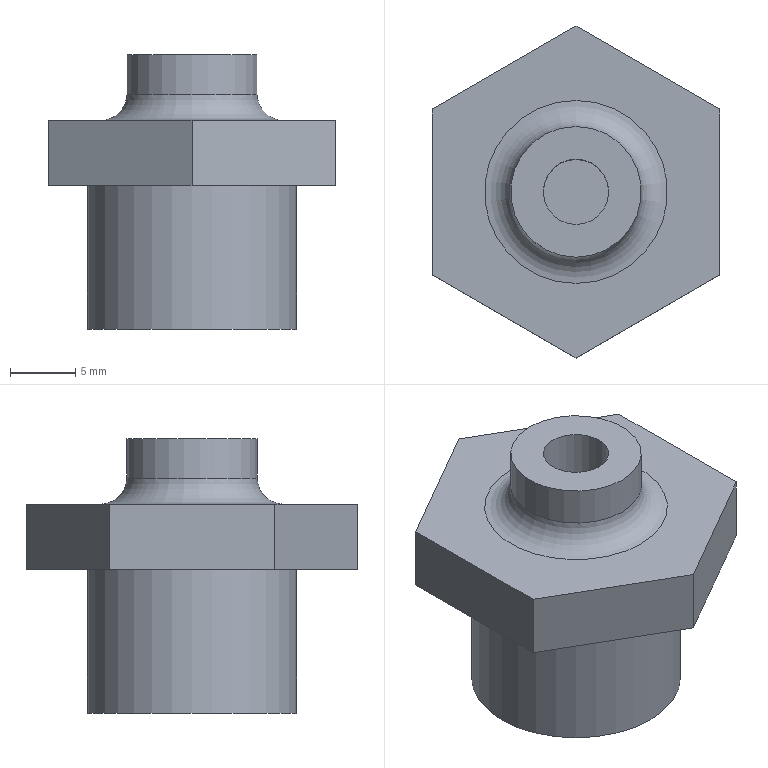Part | STEP file | 1-56.7 | 1 solid | 15 faces | box 22 x 25.403 x 21 mm | volume 4474 mm3 | plane 11 | cylinder 3 | torus 1 | commonest cylinder face diameters 5 x1 10 x1 16 x1
STEP:
#1=CARTESIAN_POINT('',(0.,0.,0.));
#2=DIRECTION('',(0.,0.,1.));
#3=DIRECTION('',(1.,0.,0.));
#4=AXIS2_PLACEMENT_3D('',#1,#2,#3);
#5=CARTESIAN_POINT('',(0.,8.,-11.));
#6=VERTEX_POINT('',#5);
#7=CARTESIAN_POINT('',(0.,0.,-11.));
#8=DIRECTION('',(0.,0.,1.));
#9=DIRECTION('',(0.,1.,0.));
#10=AXIS2_PLACEMENT_3D('',#7,#8,#9);
#11=CIRCLE('',#10,8.);
#12=CARTESIAN_POINT('',(0.,-2.144,-11.));
#13=DIRECTION('',(0.,0.,1.));
#14=DIRECTION('',(1.,0.,0.));
#15=AXIS2_PLACEMENT_3D('',#12,#13,#14);
#16=PLANE('',#15);
#17=CARTESIAN_POINT('',(0.,2.144));
#18=DIRECTION('',(0.,1.));
#19=AXIS2_PLACEMENT_2D('',#17,#18);
#20=CIRCLE('',#19,8.);
#21=(GEOMETRIC_REPRESENTATION_CONTEXT(2)PARAMETRIC_REPRESENTATION_CONTEXT()REPRESENTATION_CONTEXT('',''));
#22=DEFINITIONAL_REPRESENTATION('',(#20),#21);
#23=PCURVE('',#16,#22);
#24=CARTESIAN_POINT('',(0.,0.,0.));
#25=DIRECTION('',(0.,0.,-1.));
#26=DIRECTION('',(0.,1.,0.));
#27=AXIS2_PLACEMENT_3D('',#24,#25,#26);
#28=CYLINDRICAL_SURFACE('',#27,8.);
#29=CARTESIAN_POINT('',(6.283,11.));
#30=DIRECTION('',(-1.,0.));
#31=VECTOR('',#30,1.);
#32=LINE('',#29,#31);
#33=(GEOMETRIC_REPRESENTATION_CONTEXT(2)PARAMETRIC_REPRESENTATION_CONTEXT()REPRESENTATION_CONTEXT('',''));
#34=DEFINITIONAL_REPRESENTATION('',(#32),#33);
#35=PCURVE('',#28,#34);
#36=SURFACE_CURVE('',#11,(#23,#35),.PCURVE_S1.);
#37=EDGE_CURVE('',#6,#6,#36,.T.);
#38=ORIENTED_EDGE('',*,*,#37,.T.);
#39=EDGE_LOOP('',(#38));
#40=FACE_BOUND('',#39,.F.);
#41=ADVANCED_FACE('',(#40),#16,.F.);
#42=CARTESIAN_POINT('',(0.,8.,0.));
#43=VERTEX_POINT('',#42);
#44=CARTESIAN_POINT('',(0.,8.,0.));
#45=DIRECTION('',(0.,0.,-1.));
#46=VECTOR('',#45,1.);
#47=LINE('',#44,#46);
#48=CARTESIAN_POINT('',(6.283,0.));
#49=DIRECTION('',(0.,1.));
#50=VECTOR('',#49,1.);
#51=LINE('',#48,#50);
#52=(GEOMETRIC_REPRESENTATION_CONTEXT(2)PARAMETRIC_REPRESENTATION_CONTEXT()REPRESENTATION_CONTEXT('',''));
#53=DEFINITIONAL_REPRESENTATION('',(#51),#52);
#54=PCURVE('',#28,#53);
#55=CARTESIAN_POINT('',(0.,0.));
#56=DIRECTION('',(0.,1.));
#57=VECTOR('',#56,1.);
#58=LINE('',#55,#57);
#59=(GEOMETRIC_REPRESENTATION_CONTEXT(2)PARAMETRIC_REPRESENTATION_CONTEXT()REPRESENTATION_CONTEXT('',''));
#60=DEFINITIONAL_REPRESENTATION('',(#58),#59);
#61=PCURVE('',#28,#60);
#62=SEAM_CURVE('',#47,(#54,#61),.PCURVE_S1.);
#63=EDGE_CURVE('',#43,#6,#62,.T.);
#64=ORIENTED_EDGE('',*,*,#63,.T.);
#65=ORIENTED_EDGE('',*,*,#37,.T.);
#66=ORIENTED_EDGE('',*,*,#63,.F.);
#67=CARTESIAN_POINT('',(0.,0.,0.));
#68=DIRECTION('',(0.,0.,1.));
#69=DIRECTION('',(0.,1.,0.));
#70=AXIS2_PLACEMENT_3D('',#67,#68,#69);
#71=CIRCLE('',#70,8.);
#72=CARTESIAN_POINT('',(6.283,0.));
#73=DIRECTION('',(-1.,0.));
#74=VECTOR('',#73,1.);
#75=LINE('',#72,#74);
#76=(GEOMETRIC_REPRESENTATION_CONTEXT(2)PARAMETRIC_REPRESENTATION_CONTEXT()REPRESENTATION_CONTEXT('',''));
#77=DEFINITIONAL_REPRESENTATION('',(#75),#76);
#78=PCURVE('',#28,#77);
#79=CARTESIAN_POINT('',(1.702,0.,0.));
#80=DIRECTION('',(0.,0.,-1.));
#81=DIRECTION('',(1.,0.,0.));
#82=AXIS2_PLACEMENT_3D('',#79,#80,#81);
#83=PLANE('',#82);
#84=CARTESIAN_POINT('',(-1.702,-8.));
#85=CARTESIAN_POINT('',(-15.558,-8.));
#86=CARTESIAN_POINT('',(-8.63,4.));
#87=CARTESIAN_POINT('',(-1.702,16.));
#88=CARTESIAN_POINT('',(5.226,4.));
#89=CARTESIAN_POINT('',(12.155,-8.));
#90=CARTESIAN_POINT('',(-1.702,-8.));
#91=(BOUNDED_CURVE()B_SPLINE_CURVE(2,(#84,#85,#86,#87,#88,#89,#90),.UNSPECIFIED.,.T.,.F.)B_SPLINE_CURVE_WITH_KNOTS((1,2,2,2,2,1),(-2.094,0.,2.094,4.189,6.283,8.378),.UNSPECIFIED.)CURVE()GEOMETRIC_REPRESENTATION_ITEM()RATIONAL_B_SPLINE_CURVE((1.,0.5,1.,0.5,1.,0.5,1.))REPRESENTATION_ITEM(''));
#92=(GEOMETRIC_REPRESENTATION_CONTEXT(2)PARAMETRIC_REPRESENTATION_CONTEXT()REPRESENTATION_CONTEXT('',''));
#93=DEFINITIONAL_REPRESENTATION('',(#91),#92);
#94=PCURVE('',#83,#93);
#95=SURFACE_CURVE('',#71,(#78,#94),.PCURVE_S1.);
#96=EDGE_CURVE('',#43,#43,#95,.T.);
#97=ORIENTED_EDGE('',*,*,#96,.F.);
#98=EDGE_LOOP('',(#64,#65,#66,#97));
#99=FACE_BOUND('',#98,.T.);
#100=ADVANCED_FACE('',(#99),#28,.T.);
#101=CARTESIAN_POINT('',(-11.,-6.351,0.));
#102=VERTEX_POINT('',#101);
#103=CARTESIAN_POINT('',(-11.,6.351,0.));
#104=VERTEX_POINT('',#103);
#105=CARTESIAN_POINT('',(-11.,-6.351,0.));
#106=DIRECTION('',(0.,1.,0.));
#107=VECTOR('',#106,1.);
#108=LINE('',#105,#107);
#109=CARTESIAN_POINT('',(-12.702,6.351));
#110=DIRECTION('',(0.,-1.));
#111=VECTOR('',#110,1.);
#112=LINE('',#109,#111);
#113=(GEOMETRIC_REPRESENTATION_CONTEXT(2)PARAMETRIC_REPRESENTATION_CONTEXT()REPRESENTATION_CONTEXT('',''));
#114=DEFINITIONAL_REPRESENTATION('',(#112),#113);
#115=PCURVE('',#83,#114);
#116=CARTESIAN_POINT('',(-11.,0.,2.5));
#117=DIRECTION('',(1.,0.,0.));
#118=DIRECTION('',(0.,1.,0.));
#119=AXIS2_PLACEMENT_3D('',#116,#117,#118);
#120=PLANE('',#119);
#121=CARTESIAN_POINT('',(-6.351,-2.5));
#122=DIRECTION('',(1.,0.));
#123=VECTOR('',#122,1.);
#124=LINE('',#121,#123);
#125=(GEOMETRIC_REPRESENTATION_CONTEXT(2)PARAMETRIC_REPRESENTATION_CONTEXT()REPRESENTATION_CONTEXT('',''));
#126=DEFINITIONAL_REPRESENTATION('',(#124),#125);
#127=PCURVE('',#120,#126);
#128=SURFACE_CURVE('',#108,(#115,#127),.PCURVE_S1.);
#129=EDGE_CURVE('',#102,#104,#128,.T.);
#130=ORIENTED_EDGE('',*,*,#129,.T.);
#131=CARTESIAN_POINT('',(0.,12.702,0.));
#132=VERTEX_POINT('',#131);
#133=CARTESIAN_POINT('',(-11.,6.351,0.));
#134=DIRECTION('',(0.866,0.5,0.));
#135=VECTOR('',#134,1.);
#136=LINE('',#133,#135);
#137=CARTESIAN_POINT('',(-12.702,-6.351));
#138=DIRECTION('',(0.866,-0.5));
#139=VECTOR('',#138,1.);
#140=LINE('',#137,#139);
#141=(GEOMETRIC_REPRESENTATION_CONTEXT(2)PARAMETRIC_REPRESENTATION_CONTEXT()REPRESENTATION_CONTEXT('',''));
#142=DEFINITIONAL_REPRESENTATION('',(#140),#141);
#143=PCURVE('',#83,#142);
#144=CARTESIAN_POINT('',(-5.5,9.526,2.5));
#145=DIRECTION('',(0.5,-0.866,0.));
#146=DIRECTION('',(0.866,0.5,0.));
#147=AXIS2_PLACEMENT_3D('',#144,#145,#146);
#148=PLANE('',#147);
#149=CARTESIAN_POINT('',(-6.351,-2.5));
#150=DIRECTION('',(1.,0.));
#151=VECTOR('',#150,1.);
#152=LINE('',#149,#151);
#153=(GEOMETRIC_REPRESENTATION_CONTEXT(2)PARAMETRIC_REPRESENTATION_CONTEXT()REPRESENTATION_CONTEXT('',''));
#154=DEFINITIONAL_REPRESENTATION('',(#152),#153);
#155=PCURVE('',#148,#154);
#156=SURFACE_CURVE('',#136,(#143,#155),.PCURVE_S1.);
#157=EDGE_CURVE('',#104,#132,#156,.T.);
#158=ORIENTED_EDGE('',*,*,#157,.T.);
#159=CARTESIAN_POINT('',(11.,6.351,0.));
#160=VERTEX_POINT('',#159);
#161=CARTESIAN_POINT('',(0.,12.702,0.));
#162=DIRECTION('',(0.866,-0.5,0.));
#163=VECTOR('',#162,1.);
#164=LINE('',#161,#163);
#165=CARTESIAN_POINT('',(-1.702,-12.702));
#166=DIRECTION('',(0.866,0.5));
#167=VECTOR('',#166,1.);
#168=LINE('',#165,#167);
#169=(GEOMETRIC_REPRESENTATION_CONTEXT(2)PARAMETRIC_REPRESENTATION_CONTEXT()REPRESENTATION_CONTEXT('',''));
#170=DEFINITIONAL_REPRESENTATION('',(#168),#169);
#171=PCURVE('',#83,#170);
#172=CARTESIAN_POINT('',(5.5,9.526,2.5));
#173=DIRECTION('',(-0.5,-0.866,0.));
#174=DIRECTION('',(0.866,-0.5,0.));
#175=AXIS2_PLACEMENT_3D('',#172,#173,#174);
#176=PLANE('',#175);
#177=CARTESIAN_POINT('',(-6.351,-2.5));
#178=DIRECTION('',(1.,0.));
#179=VECTOR('',#178,1.);
#180=LINE('',#177,#179);
#181=(GEOMETRIC_REPRESENTATION_CONTEXT(2)PARAMETRIC_REPRESENTATION_CONTEXT()REPRESENTATION_CONTEXT('',''));
#182=DEFINITIONAL_REPRESENTATION('',(#180),#181);
#183=PCURVE('',#176,#182);
#184=SURFACE_CURVE('',#164,(#171,#183),.PCURVE_S1.);
#185=EDGE_CURVE('',#132,#160,#184,.T.);
#186=ORIENTED_EDGE('',*,*,#185,.T.);
#187=CARTESIAN_POINT('',(11.,-6.351,0.));
#188=VERTEX_POINT('',#187);
#189=CARTESIAN_POINT('',(11.,6.351,0.));
#190=DIRECTION('',(0.,-1.,0.));
#191=VECTOR('',#190,1.);
#192=LINE('',#189,#191);
#193=CARTESIAN_POINT('',(9.298,-6.351));
#194=DIRECTION('',(0.,1.));
#195=VECTOR('',#194,1.);
#196=LINE('',#193,#195);
#197=(GEOMETRIC_REPRESENTATION_CONTEXT(2)PARAMETRIC_REPRESENTATION_CONTEXT()REPRESENTATION_CONTEXT('',''));
#198=DEFINITIONAL_REPRESENTATION('',(#196),#197);
#199=PCURVE('',#83,#198);
#200=CARTESIAN_POINT('',(11.,0.,2.5));
#201=DIRECTION('',(-1.,0.,0.));
#202=DIRECTION('',(0.,-1.,0.));
#203=AXIS2_PLACEMENT_3D('',#200,#201,#202);
#204=PLANE('',#203);
#205=CARTESIAN_POINT('',(-6.351,-2.5));
#206=DIRECTION('',(1.,0.));
#207=VECTOR('',#206,1.);
#208=LINE('',#205,#207);
#209=(GEOMETRIC_REPRESENTATION_CONTEXT(2)PARAMETRIC_REPRESENTATION_CONTEXT()REPRESENTATION_CONTEXT('',''));
#210=DEFINITIONAL_REPRESENTATION('',(#208),#209);
#211=PCURVE('',#204,#210);
#212=SURFACE_CURVE('',#192,(#199,#211),.PCURVE_S1.);
#213=EDGE_CURVE('',#160,#188,#212,.T.);
#214=ORIENTED_EDGE('',*,*,#213,.T.);
#215=CARTESIAN_POINT('',(0.,-12.702,0.));
#216=VERTEX_POINT('',#215);
#217=CARTESIAN_POINT('',(11.,-6.351,0.));
#218=DIRECTION('',(-0.866,-0.5,0.));
#219=VECTOR('',#218,1.);
#220=LINE('',#217,#219);
#221=CARTESIAN_POINT('',(9.298,6.351));
#222=DIRECTION('',(-0.866,0.5));
#223=VECTOR('',#222,1.);
#224=LINE('',#221,#223);
#225=(GEOMETRIC_REPRESENTATION_CONTEXT(2)PARAMETRIC_REPRESENTATION_CONTEXT()REPRESENTATION_CONTEXT('',''));
#226=DEFINITIONAL_REPRESENTATION('',(#224),#225);
#227=PCURVE('',#83,#226);
#228=CARTESIAN_POINT('',(5.5,-9.526,2.5));
#229=DIRECTION('',(-0.5,0.866,0.));
#230=DIRECTION('',(-0.866,-0.5,0.));
#231=AXIS2_PLACEMENT_3D('',#228,#229,#230);
#232=PLANE('',#231);
#233=CARTESIAN_POINT('',(-6.351,-2.5));
#234=DIRECTION('',(1.,0.));
#235=VECTOR('',#234,1.);
#236=LINE('',#233,#235);
#237=(GEOMETRIC_REPRESENTATION_CONTEXT(2)PARAMETRIC_REPRESENTATION_CONTEXT()REPRESENTATION_CONTEXT('',''));
#238=DEFINITIONAL_REPRESENTATION('',(#236),#237);
#239=PCURVE('',#232,#238);
#240=SURFACE_CURVE('',#220,(#227,#239),.PCURVE_S1.);
#241=EDGE_CURVE('',#188,#216,#240,.T.);
#242=ORIENTED_EDGE('',*,*,#241,.T.);
#243=CARTESIAN_POINT('',(0.,-12.702,0.));
#244=DIRECTION('',(-0.866,0.5,0.));
#245=VECTOR('',#244,1.);
#246=LINE('',#243,#245);
#247=CARTESIAN_POINT('',(-1.702,12.702));
#248=DIRECTION('',(-0.866,-0.5));
#249=VECTOR('',#248,1.);
#250=LINE('',#247,#249);
#251=(GEOMETRIC_REPRESENTATION_CONTEXT(2)PARAMETRIC_REPRESENTATION_CONTEXT()REPRESENTATION_CONTEXT('',''));
#252=DEFINITIONAL_REPRESENTATION('',(#250),#251);
#253=PCURVE('',#83,#252);
#254=CARTESIAN_POINT('',(-5.5,-9.526,2.5));
#255=DIRECTION('',(0.5,0.866,0.));
#256=DIRECTION('',(-0.866,0.5,0.));
#257=AXIS2_PLACEMENT_3D('',#254,#255,#256);
#258=PLANE('',#257);
#259=CARTESIAN_POINT('',(-6.351,-2.5));
#260=DIRECTION('',(1.,0.));
#261=VECTOR('',#260,1.);
#262=LINE('',#259,#261);
#263=(GEOMETRIC_REPRESENTATION_CONTEXT(2)PARAMETRIC_REPRESENTATION_CONTEXT()REPRESENTATION_CONTEXT('',''));
#264=DEFINITIONAL_REPRESENTATION('',(#262),#263);
#265=PCURVE('',#258,#264);
#266=SURFACE_CURVE('',#246,(#253,#265),.PCURVE_S1.);
#267=EDGE_CURVE('',#216,#102,#266,.T.);
#268=ORIENTED_EDGE('',*,*,#267,.T.);
#269=EDGE_LOOP('',(#130,#158,#186,#214,#242,#268));
#270=FACE_BOUND('',#269,.T.);
#271=ORIENTED_EDGE('',*,*,#96,.T.);
#272=EDGE_LOOP('',(#271));
#273=FACE_BOUND('',#272,.T.);
#274=ADVANCED_FACE('',(#270,#273),#83,.T.);
#275=ORIENTED_EDGE('',*,*,#129,.T.);
#276=CARTESIAN_POINT('',(-11.,6.351,5.));
#277=VERTEX_POINT('',#276);
#278=CARTESIAN_POINT('',(-11.,6.351,0.));
#279=DIRECTION('',(0.,0.,1.));
#280=VECTOR('',#279,1.);
#281=LINE('',#278,#280);
#282=CARTESIAN_POINT('',(6.351,-2.5));
#283=DIRECTION('',(0.,1.));
#284=VECTOR('',#283,1.);
#285=LINE('',#282,#284);
#286=(GEOMETRIC_REPRESENTATION_CONTEXT(2)PARAMETRIC_REPRESENTATION_CONTEXT()REPRESENTATION_CONTEXT('',''));
#287=DEFINITIONAL_REPRESENTATION('',(#285),#286);
#288=PCURVE('',#120,#287);
#289=CARTESIAN_POINT('',(-6.351,-2.5));
#290=DIRECTION('',(0.,1.));
#291=VECTOR('',#290,1.);
#292=LINE('',#289,#291);
#293=(GEOMETRIC_REPRESENTATION_CONTEXT(2)PARAMETRIC_REPRESENTATION_CONTEXT()REPRESENTATION_CONTEXT('',''));
#294=DEFINITIONAL_REPRESENTATION('',(#292),#293);
#295=PCURVE('',#148,#294);
#296=SURFACE_CURVE('',#281,(#288,#295),.PCURVE_S1.);
#297=EDGE_CURVE('',#104,#277,#296,.T.);
#298=ORIENTED_EDGE('',*,*,#297,.T.);
#299=CARTESIAN_POINT('',(-11.,-6.351,5.));
#300=VERTEX_POINT('',#299);
#301=CARTESIAN_POINT('',(-11.,-6.351,5.));
#302=DIRECTION('',(0.,1.,0.));
#303=VECTOR('',#302,1.);
#304=LINE('',#301,#303);
#305=CARTESIAN_POINT('',(-6.351,2.5));
#306=DIRECTION('',(1.,0.));
#307=VECTOR('',#306,1.);
#308=LINE('',#305,#307);
#309=(GEOMETRIC_REPRESENTATION_CONTEXT(2)PARAMETRIC_REPRESENTATION_CONTEXT()REPRESENTATION_CONTEXT('',''));
#310=DEFINITIONAL_REPRESENTATION('',(#308),#309);
#311=PCURVE('',#120,#310);
#312=CARTESIAN_POINT('',(1.702,0.,5.));
#313=DIRECTION('',(0.,0.,-1.));
#314=DIRECTION('',(1.,0.,0.));
#315=AXIS2_PLACEMENT_3D('',#312,#313,#314);
#316=PLANE('',#315);
#317=CARTESIAN_POINT('',(-12.702,6.351));
#318=DIRECTION('',(0.,-1.));
#319=VECTOR('',#318,1.);
#320=LINE('',#317,#319);
#321=(GEOMETRIC_REPRESENTATION_CONTEXT(2)PARAMETRIC_REPRESENTATION_CONTEXT()REPRESENTATION_CONTEXT('',''));
#322=DEFINITIONAL_REPRESENTATION('',(#320),#321);
#323=PCURVE('',#316,#322);
#324=SURFACE_CURVE('',#304,(#311,#323),.PCURVE_S1.);
#325=EDGE_CURVE('',#300,#277,#324,.T.);
#326=ORIENTED_EDGE('',*,*,#325,.F.);
#327=CARTESIAN_POINT('',(-11.,-6.351,0.));
#328=DIRECTION('',(0.,0.,1.));
#329=VECTOR('',#328,1.);
#330=LINE('',#327,#329);
#331=CARTESIAN_POINT('',(-6.351,-2.5));
#332=DIRECTION('',(0.,1.));
#333=VECTOR('',#332,1.);
#334=LINE('',#331,#333);
#335=(GEOMETRIC_REPRESENTATION_CONTEXT(2)PARAMETRIC_REPRESENTATION_CONTEXT()REPRESENTATION_CONTEXT('',''));
#336=DEFINITIONAL_REPRESENTATION('',(#334),#335);
#337=PCURVE('',#120,#336);
#338=CARTESIAN_POINT('',(6.351,-2.5));
#339=DIRECTION('',(0.,1.));
#340=VECTOR('',#339,1.);
#341=LINE('',#338,#340);
#342=(GEOMETRIC_REPRESENTATION_CONTEXT(2)PARAMETRIC_REPRESENTATION_CONTEXT()REPRESENTATION_CONTEXT('',''));
#343=DEFINITIONAL_REPRESENTATION('',(#341),#342);
#344=PCURVE('',#258,#343);
#345=SURFACE_CURVE('',#330,(#337,#344),.PCURVE_S1.);
#346=EDGE_CURVE('',#102,#300,#345,.T.);
#347=ORIENTED_EDGE('',*,*,#346,.F.);
#348=EDGE_LOOP('',(#275,#298,#326,#347));
#349=FACE_BOUND('',#348,.F.);
#350=ADVANCED_FACE('',(#349),#120,.F.);
#351=ORIENTED_EDGE('',*,*,#157,.T.);
#352=CARTESIAN_POINT('',(0.,12.702,5.));
#353=VERTEX_POINT('',#352);
#354=CARTESIAN_POINT('',(0.,12.702,0.));
#355=DIRECTION('',(0.,0.,1.));
#356=VECTOR('',#355,1.);
#357=LINE('',#354,#356);
#358=CARTESIAN_POINT('',(6.351,-2.5));
#359=DIRECTION('',(0.,1.));
#360=VECTOR('',#359,1.);
#361=LINE('',#358,#360);
#362=(GEOMETRIC_REPRESENTATION_CONTEXT(2)PARAMETRIC_REPRESENTATION_CONTEXT()REPRESENTATION_CONTEXT('',''));
#363=DEFINITIONAL_REPRESENTATION('',(#361),#362);
#364=PCURVE('',#148,#363);
#365=CARTESIAN_POINT('',(-6.351,-2.5));
#366=DIRECTION('',(0.,1.));
#367=VECTOR('',#366,1.);
#368=LINE('',#365,#367);
#369=(GEOMETRIC_REPRESENTATION_CONTEXT(2)PARAMETRIC_REPRESENTATION_CONTEXT()REPRESENTATION_CONTEXT('',''));
#370=DEFINITIONAL_REPRESENTATION('',(#368),#369);
#371=PCURVE('',#176,#370);
#372=SURFACE_CURVE('',#357,(#364,#371),.PCURVE_S1.);
#373=EDGE_CURVE('',#132,#353,#372,.T.);
#374=ORIENTED_EDGE('',*,*,#373,.T.);
#375=CARTESIAN_POINT('',(-11.,6.351,5.));
#376=DIRECTION('',(0.866,0.5,0.));
#377=VECTOR('',#376,1.);
#378=LINE('',#375,#377);
#379=CARTESIAN_POINT('',(-6.351,2.5));
#380=DIRECTION('',(1.,0.));
#381=VECTOR('',#380,1.);
#382=LINE('',#379,#381);
#383=(GEOMETRIC_REPRESENTATION_CONTEXT(2)PARAMETRIC_REPRESENTATION_CONTEXT()REPRESENTATION_CONTEXT('',''));
#384=DEFINITIONAL_REPRESENTATION('',(#382),#383);
#385=PCURVE('',#148,#384);
#386=CARTESIAN_POINT('',(-12.702,-6.351));
#387=DIRECTION('',(0.866,-0.5));
#388=VECTOR('',#387,1.);
#389=LINE('',#386,#388);
#390=(GEOMETRIC_REPRESENTATION_CONTEXT(2)PARAMETRIC_REPRESENTATION_CONTEXT()REPRESENTATION_CONTEXT('',''));
#391=DEFINITIONAL_REPRESENTATION('',(#389),#390);
#392=PCURVE('',#316,#391);
#393=SURFACE_CURVE('',#378,(#385,#392),.PCURVE_S1.);
#394=EDGE_CURVE('',#277,#353,#393,.T.);
#395=ORIENTED_EDGE('',*,*,#394,.F.);
#396=ORIENTED_EDGE('',*,*,#297,.F.);
#397=EDGE_LOOP('',(#351,#374,#395,#396));
#398=FACE_BOUND('',#397,.F.);
#399=ADVANCED_FACE('',(#398),#148,.F.);
#400=ORIENTED_EDGE('',*,*,#185,.T.);
#401=CARTESIAN_POINT('',(11.,6.351,5.));
#402=VERTEX_POINT('',#401);
#403=CARTESIAN_POINT('',(11.,6.351,0.));
#404=DIRECTION('',(0.,0.,1.));
#405=VECTOR('',#404,1.);
#406=LINE('',#403,#405);
#407=CARTESIAN_POINT('',(6.351,-2.5));
#408=DIRECTION('',(0.,1.));
#409=VECTOR('',#408,1.);
#410=LINE('',#407,#409);
#411=(GEOMETRIC_REPRESENTATION_CONTEXT(2)PARAMETRIC_REPRESENTATION_CONTEXT()REPRESENTATION_CONTEXT('',''));
#412=DEFINITIONAL_REPRESENTATION('',(#410),#411);
#413=PCURVE('',#176,#412);
#414=CARTESIAN_POINT('',(-6.351,-2.5));
#415=DIRECTION('',(0.,1.));
#416=VECTOR('',#415,1.);
#417=LINE('',#414,#416);
#418=(GEOMETRIC_REPRESENTATION_CONTEXT(2)PARAMETRIC_REPRESENTATION_CONTEXT()REPRESENTATION_CONTEXT('',''));
#419=DEFINITIONAL_REPRESENTATION('',(#417),#418);
#420=PCURVE('',#204,#419);
#421=SURFACE_CURVE('',#406,(#413,#420),.PCURVE_S1.);
#422=EDGE_CURVE('',#160,#402,#421,.T.);
#423=ORIENTED_EDGE('',*,*,#422,.T.);
#424=CARTESIAN_POINT('',(0.,12.702,5.));
#425=DIRECTION('',(0.866,-0.5,0.));
#426=VECTOR('',#425,1.);
#427=LINE('',#424,#426);
#428=CARTESIAN_POINT('',(-6.351,2.5));
#429=DIRECTION('',(1.,0.));
#430=VECTOR('',#429,1.);
#431=LINE('',#428,#430);
#432=(GEOMETRIC_REPRESENTATION_CONTEXT(2)PARAMETRIC_REPRESENTATION_CONTEXT()REPRESENTATION_CONTEXT('',''));
#433=DEFINITIONAL_REPRESENTATION('',(#431),#432);
#434=PCURVE('',#176,#433);
#435=CARTESIAN_POINT('',(-1.702,-12.702));
#436=DIRECTION('',(0.866,0.5));
#437=VECTOR('',#436,1.);
#438=LINE('',#435,#437);
#439=(GEOMETRIC_REPRESENTATION_CONTEXT(2)PARAMETRIC_REPRESENTATION_CONTEXT()REPRESENTATION_CONTEXT('',''));
#440=DEFINITIONAL_REPRESENTATION('',(#438),#439);
#441=PCURVE('',#316,#440);
#442=SURFACE_CURVE('',#427,(#434,#441),.PCURVE_S1.);
#443=EDGE_CURVE('',#353,#402,#442,.T.);
#444=ORIENTED_EDGE('',*,*,#443,.F.);
#445=ORIENTED_EDGE('',*,*,#373,.F.);
#446=EDGE_LOOP('',(#400,#423,#444,#445));
#447=FACE_BOUND('',#446,.F.);
#448=ADVANCED_FACE('',(#447),#176,.F.);
#449=ORIENTED_EDGE('',*,*,#213,.T.);
#450=CARTESIAN_POINT('',(11.,-6.351,5.));
#451=VERTEX_POINT('',#450);
#452=CARTESIAN_POINT('',(11.,-6.351,0.));
#453=DIRECTION('',(0.,0.,1.));
#454=VECTOR('',#453,1.);
#455=LINE('',#452,#454);
#456=CARTESIAN_POINT('',(6.351,-2.5));
#457=DIRECTION('',(0.,1.));
#458=VECTOR('',#457,1.);
#459=LINE('',#456,#458);
#460=(GEOMETRIC_REPRESENTATION_CONTEXT(2)PARAMETRIC_REPRESENTATION_CONTEXT()REPRESENTATION_CONTEXT('',''));
#461=DEFINITIONAL_REPRESENTATION('',(#459),#460);
#462=PCURVE('',#204,#461);
#463=CARTESIAN_POINT('',(-6.351,-2.5));
#464=DIRECTION('',(0.,1.));
#465=VECTOR('',#464,1.);
#466=LINE('',#463,#465);
#467=(GEOMETRIC_REPRESENTATION_CONTEXT(2)PARAMETRIC_REPRESENTATION_CONTEXT()REPRESENTATION_CONTEXT('',''));
#468=DEFINITIONAL_REPRESENTATION('',(#466),#467);
#469=PCURVE('',#232,#468);
#470=SURFACE_CURVE('',#455,(#462,#469),.PCURVE_S1.);
#471=EDGE_CURVE('',#188,#451,#470,.T.);
#472=ORIENTED_EDGE('',*,*,#471,.T.);
#473=CARTESIAN_POINT('',(11.,6.351,5.));
#474=DIRECTION('',(0.,-1.,0.));
#475=VECTOR('',#474,1.);
#476=LINE('',#473,#475);
#477=CARTESIAN_POINT('',(-6.351,2.5));
#478=DIRECTION('',(1.,0.));
#479=VECTOR('',#478,1.);
#480=LINE('',#477,#479);
#481=(GEOMETRIC_REPRESENTATION_CONTEXT(2)PARAMETRIC_REPRESENTATION_CONTEXT()REPRESENTATION_CONTEXT('',''));
#482=DEFINITIONAL_REPRESENTATION('',(#480),#481);
#483=PCURVE('',#204,#482);
#484=CARTESIAN_POINT('',(9.298,-6.351));
#485=DIRECTION('',(0.,1.));
#486=VECTOR('',#485,1.);
#487=LINE('',#484,#486);
#488=(GEOMETRIC_REPRESENTATION_CONTEXT(2)PARAMETRIC_REPRESENTATION_CONTEXT()REPRESENTATION_CONTEXT('',''));
#489=DEFINITIONAL_REPRESENTATION('',(#487),#488);
#490=PCURVE('',#316,#489);
#491=SURFACE_CURVE('',#476,(#483,#490),.PCURVE_S1.);
#492=EDGE_CURVE('',#402,#451,#491,.T.);
#493=ORIENTED_EDGE('',*,*,#492,.F.);
#494=ORIENTED_EDGE('',*,*,#422,.F.);
#495=EDGE_LOOP('',(#449,#472,#493,#494));
#496=FACE_BOUND('',#495,.F.);
#497=ADVANCED_FACE('',(#496),#204,.F.);
#498=ORIENTED_EDGE('',*,*,#241,.T.);
#499=CARTESIAN_POINT('',(0.,-12.702,5.));
#500=VERTEX_POINT('',#499);
#501=CARTESIAN_POINT('',(0.,-12.702,0.));
#502=DIRECTION('',(0.,0.,1.));
#503=VECTOR('',#502,1.);
#504=LINE('',#501,#503);
#505=CARTESIAN_POINT('',(6.351,-2.5));
#506=DIRECTION('',(0.,1.));
#507=VECTOR('',#506,1.);
#508=LINE('',#505,#507);
#509=(GEOMETRIC_REPRESENTATION_CONTEXT(2)PARAMETRIC_REPRESENTATION_CONTEXT()REPRESENTATION_CONTEXT('',''));
#510=DEFINITIONAL_REPRESENTATION('',(#508),#509);
#511=PCURVE('',#232,#510);
#512=CARTESIAN_POINT('',(-6.351,-2.5));
#513=DIRECTION('',(0.,1.));
#514=VECTOR('',#513,1.);
#515=LINE('',#512,#514);
#516=(GEOMETRIC_REPRESENTATION_CONTEXT(2)PARAMETRIC_REPRESENTATION_CONTEXT()REPRESENTATION_CONTEXT('',''));
#517=DEFINITIONAL_REPRESENTATION('',(#515),#516);
#518=PCURVE('',#258,#517);
#519=SURFACE_CURVE('',#504,(#511,#518),.PCURVE_S1.);
#520=EDGE_CURVE('',#216,#500,#519,.T.);
#521=ORIENTED_EDGE('',*,*,#520,.T.);
#522=CARTESIAN_POINT('',(11.,-6.351,5.));
#523=DIRECTION('',(-0.866,-0.5,0.));
#524=VECTOR('',#523,1.);
#525=LINE('',#522,#524);
#526=CARTESIAN_POINT('',(-6.351,2.5));
#527=DIRECTION('',(1.,0.));
#528=VECTOR('',#527,1.);
#529=LINE('',#526,#528);
#530=(GEOMETRIC_REPRESENTATION_CONTEXT(2)PARAMETRIC_REPRESENTATION_CONTEXT()REPRESENTATION_CONTEXT('',''));
#531=DEFINITIONAL_REPRESENTATION('',(#529),#530);
#532=PCURVE('',#232,#531);
#533=CARTESIAN_POINT('',(9.298,6.351));
#534=DIRECTION('',(-0.866,0.5));
#535=VECTOR('',#534,1.);
#536=LINE('',#533,#535);
#537=(GEOMETRIC_REPRESENTATION_CONTEXT(2)PARAMETRIC_REPRESENTATION_CONTEXT()REPRESENTATION_CONTEXT('',''));
#538=DEFINITIONAL_REPRESENTATION('',(#536),#537);
#539=PCURVE('',#316,#538);
#540=SURFACE_CURVE('',#525,(#532,#539),.PCURVE_S1.);
#541=EDGE_CURVE('',#451,#500,#540,.T.);
#542=ORIENTED_EDGE('',*,*,#541,.F.);
#543=ORIENTED_EDGE('',*,*,#471,.F.);
#544=EDGE_LOOP('',(#498,#521,#542,#543));
#545=FACE_BOUND('',#544,.F.);
#546=ADVANCED_FACE('',(#545),#232,.F.);
#547=ORIENTED_EDGE('',*,*,#267,.T.);
#548=ORIENTED_EDGE('',*,*,#346,.T.);
#549=CARTESIAN_POINT('',(0.,-12.702,5.));
#550=DIRECTION('',(-0.866,0.5,0.));
#551=VECTOR('',#550,1.);
#552=LINE('',#549,#551);
#553=CARTESIAN_POINT('',(-6.351,2.5));
#554=DIRECTION('',(1.,0.));
#555=VECTOR('',#554,1.);
#556=LINE('',#553,#555);
#557=(GEOMETRIC_REPRESENTATION_CONTEXT(2)PARAMETRIC_REPRESENTATION_CONTEXT()REPRESENTATION_CONTEXT('',''));
#558=DEFINITIONAL_REPRESENTATION('',(#556),#557);
#559=PCURVE('',#258,#558);
#560=CARTESIAN_POINT('',(-1.702,12.702));
#561=DIRECTION('',(-0.866,-0.5));
#562=VECTOR('',#561,1.);
#563=LINE('',#560,#562);
#564=(GEOMETRIC_REPRESENTATION_CONTEXT(2)PARAMETRIC_REPRESENTATION_CONTEXT()REPRESENTATION_CONTEXT('',''));
#565=DEFINITIONAL_REPRESENTATION('',(#563),#564);
#566=PCURVE('',#316,#565);
#567=SURFACE_CURVE('',#552,(#559,#566),.PCURVE_S1.);
#568=EDGE_CURVE('',#500,#300,#567,.T.);
#569=ORIENTED_EDGE('',*,*,#568,.F.);
#570=ORIENTED_EDGE('',*,*,#520,.F.);
#571=EDGE_LOOP('',(#547,#548,#569,#570));
#572=FACE_BOUND('',#571,.F.);
#573=ADVANCED_FACE('',(#572),#258,.F.);
#574=CARTESIAN_POINT('',(0.,5.,10.));
#575=VERTEX_POINT('',#574);
#576=CARTESIAN_POINT('',(0.,0.,10.));
#577=DIRECTION('',(0.,0.,1.));
#578=DIRECTION('',(0.,1.,0.));
#579=AXIS2_PLACEMENT_3D('',#576,#577,#578);
#580=CIRCLE('',#579,5.);
#581=CARTESIAN_POINT('',(0.,-1.34,10.));
#582=DIRECTION('',(0.,0.,1.));
#583=DIRECTION('',(1.,0.,0.));
#584=AXIS2_PLACEMENT_3D('',#581,#582,#583);
#585=PLANE('',#584);
#586=CARTESIAN_POINT('',(0.,1.34));
#587=DIRECTION('',(0.,1.));
#588=AXIS2_PLACEMENT_2D('',#586,#587);
#589=CIRCLE('',#588,5.);
#590=(GEOMETRIC_REPRESENTATION_CONTEXT(2)PARAMETRIC_REPRESENTATION_CONTEXT()REPRESENTATION_CONTEXT('',''));
#591=DEFINITIONAL_REPRESENTATION('',(#589),#590);
#592=PCURVE('',#585,#591);
#593=CARTESIAN_POINT('',(0.,0.,5.));
#594=DIRECTION('',(0.,0.,1.));
#595=DIRECTION('',(0.,1.,0.));
#596=AXIS2_PLACEMENT_3D('',#593,#594,#595);
#597=CYLINDRICAL_SURFACE('',#596,5.);
#598=CARTESIAN_POINT('',(0.,5.));
#599=DIRECTION('',(1.,0.));
#600=VECTOR('',#599,1.);
#601=LINE('',#598,#600);
#602=(GEOMETRIC_REPRESENTATION_CONTEXT(2)PARAMETRIC_REPRESENTATION_CONTEXT()REPRESENTATION_CONTEXT('',''));
#603=DEFINITIONAL_REPRESENTATION('',(#601),#602);
#604=PCURVE('',#597,#603);
#605=SURFACE_CURVE('',#580,(#592,#604),.PCURVE_S1.);
#606=EDGE_CURVE('',#575,#575,#605,.T.);
#607=ORIENTED_EDGE('',*,*,#606,.T.);
#608=EDGE_LOOP('',(#607));
#609=FACE_BOUND('',#608,.T.);
#610=CARTESIAN_POINT('',(0.,2.5,10.));
#611=VERTEX_POINT('',#610);
#612=CARTESIAN_POINT('',(0.,0.,10.));
#613=DIRECTION('',(0.,0.,1.));
#614=DIRECTION('',(0.,1.,0.));
#615=AXIS2_PLACEMENT_3D('',#612,#613,#614);
#616=CIRCLE('',#615,2.5);
#617=CARTESIAN_POINT('',(0.,1.34));
#618=DIRECTION('',(0.,1.));
#619=AXIS2_PLACEMENT_2D('',#617,#618);
#620=CIRCLE('',#619,2.5);
#621=(GEOMETRIC_REPRESENTATION_CONTEXT(2)PARAMETRIC_REPRESENTATION_CONTEXT()REPRESENTATION_CONTEXT('',''));
#622=DEFINITIONAL_REPRESENTATION('',(#620),#621);
#623=PCURVE('',#585,#622);
#624=CARTESIAN_POINT('',(0.,0.,10.));
#625=DIRECTION('',(0.,0.,-1.));
#626=DIRECTION('',(0.,1.,0.));
#627=AXIS2_PLACEMENT_3D('',#624,#625,#626);
#628=CYLINDRICAL_SURFACE('',#627,2.5);
#629=CARTESIAN_POINT('',(6.283,0.));
#630=DIRECTION('',(-1.,0.));
#631=VECTOR('',#630,1.);
#632=LINE('',#629,#631);
#633=(GEOMETRIC_REPRESENTATION_CONTEXT(2)PARAMETRIC_REPRESENTATION_CONTEXT()REPRESENTATION_CONTEXT('',''));
#634=DEFINITIONAL_REPRESENTATION('',(#632),#633);
#635=PCURVE('',#628,#634);
#636=SURFACE_CURVE('',#616,(#623,#635),.PCURVE_S1.);
#637=EDGE_CURVE('',#611,#611,#636,.T.);
#638=ORIENTED_EDGE('',*,*,#637,.F.);
#639=EDGE_LOOP('',(#638));
#640=FACE_BOUND('',#639,.T.);
#641=ADVANCED_FACE('',(#609,#640),#585,.T.);
#642=CARTESIAN_POINT('',(0.,2.5,-3.));
#643=VERTEX_POINT('',#642);
#644=CARTESIAN_POINT('',(0.,2.5,10.));
#645=DIRECTION('',(0.,0.,-1.));
#646=VECTOR('',#645,1.);
#647=LINE('',#644,#646);
#648=CARTESIAN_POINT('',(6.283,0.));
#649=DIRECTION('',(0.,1.));
#650=VECTOR('',#649,1.);
#651=LINE('',#648,#650);
#652=(GEOMETRIC_REPRESENTATION_CONTEXT(2)PARAMETRIC_REPRESENTATION_CONTEXT()REPRESENTATION_CONTEXT('',''));
#653=DEFINITIONAL_REPRESENTATION('',(#651),#652);
#654=PCURVE('',#628,#653);
#655=CARTESIAN_POINT('',(0.,0.));
#656=DIRECTION('',(0.,1.));
#657=VECTOR('',#656,1.);
#658=LINE('',#655,#657);
#659=(GEOMETRIC_REPRESENTATION_CONTEXT(2)PARAMETRIC_REPRESENTATION_CONTEXT()REPRESENTATION_CONTEXT('',''));
#660=DEFINITIONAL_REPRESENTATION('',(#658),#659);
#661=PCURVE('',#628,#660);
#662=SEAM_CURVE('',#647,(#654,#661),.PCURVE_S1.);
#663=EDGE_CURVE('',#611,#643,#662,.T.);
#664=ORIENTED_EDGE('',*,*,#663,.T.);
#665=CARTESIAN_POINT('',(0.,0.,-3.));
#666=DIRECTION('',(0.,0.,1.));
#667=DIRECTION('',(0.,1.,0.));
#668=AXIS2_PLACEMENT_3D('',#665,#666,#667);
#669=CIRCLE('',#668,2.5);
#670=CARTESIAN_POINT('',(6.283,13.));
#671=DIRECTION('',(-1.,0.));
#672=VECTOR('',#671,1.);
#673=LINE('',#670,#672);
#674=(GEOMETRIC_REPRESENTATION_CONTEXT(2)PARAMETRIC_REPRESENTATION_CONTEXT()REPRESENTATION_CONTEXT('',''));
#675=DEFINITIONAL_REPRESENTATION('',(#673),#674);
#676=PCURVE('',#628,#675);
#677=CARTESIAN_POINT('',(0.,-0.6699,-3.));
#678=DIRECTION('',(0.,0.,1.));
#679=DIRECTION('',(1.,0.,0.));
#680=AXIS2_PLACEMENT_3D('',#677,#678,#679);
#681=PLANE('',#680);
#682=CARTESIAN_POINT('',(0.,0.6699));
#683=DIRECTION('',(0.,1.));
#684=AXIS2_PLACEMENT_2D('',#682,#683);
#685=CIRCLE('',#684,2.5);
#686=(GEOMETRIC_REPRESENTATION_CONTEXT(2)PARAMETRIC_REPRESENTATION_CONTEXT()REPRESENTATION_CONTEXT('',''));
#687=DEFINITIONAL_REPRESENTATION('',(#685),#686);
#688=PCURVE('',#681,#687);
#689=SURFACE_CURVE('',#669,(#676,#688),.PCURVE_S1.);
#690=EDGE_CURVE('',#643,#643,#689,.T.);
#691=ORIENTED_EDGE('',*,*,#690,.T.);
#692=ORIENTED_EDGE('',*,*,#663,.F.);
#693=ORIENTED_EDGE('',*,*,#637,.F.);
#694=EDGE_LOOP('',(#664,#691,#692,#693));
#695=FACE_BOUND('',#694,.F.);
#696=ADVANCED_FACE('',(#695),#628,.F.);
#697=ORIENTED_EDGE('',*,*,#690,.T.);
#698=EDGE_LOOP('',(#697));
#699=FACE_BOUND('',#698,.T.);
#700=ADVANCED_FACE('',(#699),#681,.T.);
#701=ORIENTED_EDGE('',*,*,#325,.T.);
#702=ORIENTED_EDGE('',*,*,#394,.T.);
#703=ORIENTED_EDGE('',*,*,#443,.T.);
#704=ORIENTED_EDGE('',*,*,#492,.T.);
#705=ORIENTED_EDGE('',*,*,#541,.T.);
#706=ORIENTED_EDGE('',*,*,#568,.T.);
#707=EDGE_LOOP('',(#701,#702,#703,#704,#705,#706));
#708=FACE_BOUND('',#707,.F.);
#709=CARTESIAN_POINT('',(0.,7.,5.));
#710=VERTEX_POINT('',#709);
#711=CARTESIAN_POINT('',(0.,0.,5.));
#712=DIRECTION('',(0.,0.,-1.));
#713=DIRECTION('',(0.,1.,0.));
#714=AXIS2_PLACEMENT_3D('',#711,#712,#713);
#715=CIRCLE('',#714,7.);
#716=CARTESIAN_POINT('',(-1.702,0.));
#717=DIRECTION('',(0.,-1.));
#718=AXIS2_PLACEMENT_2D('',#716,#717);
#719=CIRCLE('',#718,7.);
#720=(GEOMETRIC_REPRESENTATION_CONTEXT(2)PARAMETRIC_REPRESENTATION_CONTEXT()REPRESENTATION_CONTEXT('',''));
#721=DEFINITIONAL_REPRESENTATION('',(#719),#720);
#722=PCURVE('',#316,#721);
#723=CARTESIAN_POINT('',(0.,0.,7.));
#724=DIRECTION('',(0.,0.,1.));
#725=DIRECTION('',(0.,1.,0.));
#726=AXIS2_PLACEMENT_3D('',#723,#724,#725);
#727=TOROIDAL_SURFACE('',#726,7.,2.);
#728=CARTESIAN_POINT('',(6.283,4.712));
#729=DIRECTION('',(-1.,0.));
#730=VECTOR('',#729,1.);
#731=LINE('',#728,#730);
#732=(GEOMETRIC_REPRESENTATION_CONTEXT(2)PARAMETRIC_REPRESENTATION_CONTEXT()REPRESENTATION_CONTEXT('',''));
#733=DEFINITIONAL_REPRESENTATION('',(#731),#732);
#734=PCURVE('',#727,#733);
#735=SURFACE_CURVE('',#715,(#722,#734),.PCURVE_S1.);
#736=EDGE_CURVE('',#710,#710,#735,.T.);
#737=ORIENTED_EDGE('',*,*,#736,.F.);
#738=EDGE_LOOP('',(#737));
#739=FACE_BOUND('',#738,.F.);
#740=ADVANCED_FACE('',(#708,#739),#316,.F.);
#741=ORIENTED_EDGE('',*,*,#606,.F.);
#742=CARTESIAN_POINT('',(0.,5.,7.));
#743=VERTEX_POINT('',#742);
#744=CARTESIAN_POINT('',(0.,5.,7.));
#745=DIRECTION('',(0.,0.,1.));
#746=VECTOR('',#745,1.);
#747=LINE('',#744,#746);
#748=CARTESIAN_POINT('',(0.,2.));
#749=DIRECTION('',(0.,1.));
#750=VECTOR('',#749,1.);
#751=LINE('',#748,#750);
#752=(GEOMETRIC_REPRESENTATION_CONTEXT(2)PARAMETRIC_REPRESENTATION_CONTEXT()REPRESENTATION_CONTEXT('',''));
#753=DEFINITIONAL_REPRESENTATION('',(#751),#752);
#754=PCURVE('',#597,#753);
#755=CARTESIAN_POINT('',(6.283,2.));
#756=DIRECTION('',(0.,1.));
#757=VECTOR('',#756,1.);
#758=LINE('',#755,#757);
#759=(GEOMETRIC_REPRESENTATION_CONTEXT(2)PARAMETRIC_REPRESENTATION_CONTEXT()REPRESENTATION_CONTEXT('',''));
#760=DEFINITIONAL_REPRESENTATION('',(#758),#759);
#761=PCURVE('',#597,#760);
#762=SEAM_CURVE('',#747,(#754,#761),.PCURVE_S1.);
#763=EDGE_CURVE('',#743,#575,#762,.T.);
#764=ORIENTED_EDGE('',*,*,#763,.F.);
#765=CARTESIAN_POINT('',(0.,0.,7.));
#766=DIRECTION('',(0.,0.,-1.));
#767=DIRECTION('',(0.,1.,0.));
#768=AXIS2_PLACEMENT_3D('',#765,#766,#767);
#769=CIRCLE('',#768,5.);
#770=CARTESIAN_POINT('',(6.283,2.));
#771=DIRECTION('',(-1.,0.));
#772=VECTOR('',#771,1.);
#773=LINE('',#770,#772);
#774=(GEOMETRIC_REPRESENTATION_CONTEXT(2)PARAMETRIC_REPRESENTATION_CONTEXT()REPRESENTATION_CONTEXT('',''));
#775=DEFINITIONAL_REPRESENTATION('',(#773),#774);
#776=PCURVE('',#597,#775);
#777=CARTESIAN_POINT('',(6.283,3.142));
#778=DIRECTION('',(-1.,0.));
#779=VECTOR('',#778,1.);
#780=LINE('',#777,#779);
#781=(GEOMETRIC_REPRESENTATION_CONTEXT(2)PARAMETRIC_REPRESENTATION_CONTEXT()REPRESENTATION_CONTEXT('',''));
#782=DEFINITIONAL_REPRESENTATION('',(#780),#781);
#783=PCURVE('',#727,#782);
#784=SURFACE_CURVE('',#769,(#776,#783),.PCURVE_S1.);
#785=EDGE_CURVE('',#743,#743,#784,.T.);
#786=ORIENTED_EDGE('',*,*,#785,.F.);
#787=ORIENTED_EDGE('',*,*,#763,.T.);
#788=EDGE_LOOP('',(#741,#764,#786,#787));
#789=FACE_BOUND('',#788,.T.);
#790=ADVANCED_FACE('',(#789),#597,.T.);
#791=CARTESIAN_POINT('',(0.,7.,7.));
#792=DIRECTION('',(1.,0.,0.));
#793=DIRECTION('',(0.,-1.,0.));
#794=AXIS2_PLACEMENT_3D('',#791,#792,#793);
#795=CIRCLE('',#794,2.);
#796=CARTESIAN_POINT('',(0.,3.142));
#797=CARTESIAN_POINT('',(0.,3.165));
#798=CARTESIAN_POINT('',(0.,3.213));
#799=CARTESIAN_POINT('',(0.,3.284));
#800=CARTESIAN_POINT('',(0.,3.356));
#801=CARTESIAN_POINT('',(0.,3.427));
#802=CARTESIAN_POINT('',(0.,3.499));
#803=CARTESIAN_POINT('',(0.,3.57));
#804=CARTESIAN_POINT('',(0.,3.641));
#805=CARTESIAN_POINT('',(0.,3.713));
#806=CARTESIAN_POINT('',(0.,3.784));
#807=CARTESIAN_POINT('',(0.,3.856));
#808=CARTESIAN_POINT('',(0.,3.927));
#809=CARTESIAN_POINT('',(0.,3.998));
#810=CARTESIAN_POINT('',(0.,4.07));
#811=CARTESIAN_POINT('',(0.,4.141));
#812=CARTESIAN_POINT('',(0.,4.213));
#813=CARTESIAN_POINT('',(0.,4.284));
#814=CARTESIAN_POINT('',(0.,4.355));
#815=CARTESIAN_POINT('',(0.,4.427));
#816=CARTESIAN_POINT('',(0.,4.498));
#817=CARTESIAN_POINT('',(0.,4.57));
#818=CARTESIAN_POINT('',(0.,4.641));
#819=CARTESIAN_POINT('',(0.,4.689));
#820=CARTESIAN_POINT('',(0.,4.712));
#821=B_SPLINE_CURVE_WITH_KNOTS('',3,(#796,#797,#798,#799,#800,#801,#802,#803,#804,#805,#806,#807,#808,#809,#810,#811,#812,#813,#814,#815,#816,#817,#818,#819,#820),.UNSPECIFIED.,.F.,.F.,(4,1,1,1,1,1,1,1,1,1,1,1,1,1,1,1,1,1,1,1,1,1,4),(0.,0.0714,0.1428,0.2142,0.2856,0.357,0.4284,0.4998,0.5712,0.6426,0.714,0.7854,0.8568,0.9282,0.9996,1.071,1.142,1.214,1.285,1.357,1.428,1.499,1.571),.QUASI_UNIFORM_KNOTS.);
#822=(GEOMETRIC_REPRESENTATION_CONTEXT(2)PARAMETRIC_REPRESENTATION_CONTEXT()REPRESENTATION_CONTEXT('',''));
#823=DEFINITIONAL_REPRESENTATION('',(#821),#822);
#824=PCURVE('',#727,#823);
#825=CARTESIAN_POINT('',(6.283,3.142));
#826=CARTESIAN_POINT('',(6.283,3.165));
#827=CARTESIAN_POINT('',(6.283,3.213));
#828=CARTESIAN_POINT('',(6.283,3.284));
#829=CARTESIAN_POINT('',(6.283,3.356));
#830=CARTESIAN_POINT('',(6.283,3.427));
#831=CARTESIAN_POINT('',(6.283,3.499));
#832=CARTESIAN_POINT('',(6.283,3.57));
#833=CARTESIAN_POINT('',(6.283,3.641));
#834=CARTESIAN_POINT('',(6.283,3.713));
#835=CARTESIAN_POINT('',(6.283,3.784));
#836=CARTESIAN_POINT('',(6.283,3.856));
#837=CARTESIAN_POINT('',(6.283,3.927));
#838=CARTESIAN_POINT('',(6.283,3.998));
#839=CARTESIAN_POINT('',(6.283,4.07));
#840=CARTESIAN_POINT('',(6.283,4.141));
#841=CARTESIAN_POINT('',(6.283,4.213));
#842=CARTESIAN_POINT('',(6.283,4.284));
#843=CARTESIAN_POINT('',(6.283,4.355));
#844=CARTESIAN_POINT('',(6.283,4.427));
#845=CARTESIAN_POINT('',(6.283,4.498));
#846=CARTESIAN_POINT('',(6.283,4.57));
#847=CARTESIAN_POINT('',(6.283,4.641));
#848=CARTESIAN_POINT('',(6.283,4.689));
#849=CARTESIAN_POINT('',(6.283,4.712));
#850=B_SPLINE_CURVE_WITH_KNOTS('',3,(#825,#826,#827,#828,#829,#830,#831,#832,#833,#834,#835,#836,#837,#838,#839,#840,#841,#842,#843,#844,#845,#846,#847,#848,#849),.UNSPECIFIED.,.F.,.F.,(4,1,1,1,1,1,1,1,1,1,1,1,1,1,1,1,1,1,1,1,1,1,4),(0.,0.0714,0.1428,0.2142,0.2856,0.357,0.4284,0.4998,0.5712,0.6426,0.714,0.7854,0.8568,0.9282,0.9996,1.071,1.142,1.214,1.285,1.357,1.428,1.499,1.571),.QUASI_UNIFORM_KNOTS.);
#851=(GEOMETRIC_REPRESENTATION_CONTEXT(2)PARAMETRIC_REPRESENTATION_CONTEXT()REPRESENTATION_CONTEXT('',''));
#852=DEFINITIONAL_REPRESENTATION('',(#850),#851);
#853=PCURVE('',#727,#852);
#854=SEAM_CURVE('',#795,(#824,#853),.PCURVE_S1.);
#855=EDGE_CURVE('',#743,#710,#854,.T.);
#856=ORIENTED_EDGE('',*,*,#855,.F.);
#857=ORIENTED_EDGE('',*,*,#785,.F.);
#858=ORIENTED_EDGE('',*,*,#855,.T.);
#859=ORIENTED_EDGE('',*,*,#736,.T.);
#860=EDGE_LOOP('',(#856,#857,#858,#859));
#861=FACE_BOUND('',#860,.F.);
#862=ADVANCED_FACE('',(#861),#727,.F.);
#863=CLOSED_SHELL('',(#41,#100,#274,#350,#399,#448,#497,#546,#573,#641,#696,#700,#740,#790,#862));
#864=MANIFOLD_SOLID_BREP('',#863);
#865=(LENGTH_UNIT()NAMED_UNIT(*)SI_UNIT(.MILLI.,.METRE.));
#866=UNCERTAINTY_MEASURE_WITH_UNIT(LENGTH_MEASURE(0.0000001),#865,'','');
#867=(NAMED_UNIT(*)PLANE_ANGLE_UNIT()SI_UNIT($,.RADIAN.));
#868=(NAMED_UNIT(*)SI_UNIT($,.STERADIAN.)SOLID_ANGLE_UNIT());
#869=(GEOMETRIC_REPRESENTATION_CONTEXT(3)GLOBAL_UNCERTAINTY_ASSIGNED_CONTEXT((#866))GLOBAL_UNIT_ASSIGNED_CONTEXT((#865,#867,#868))REPRESENTATION_CONTEXT('',''));
#870=ADVANCED_BREP_SHAPE_REPRESENTATION('',(#4,#864),#869);